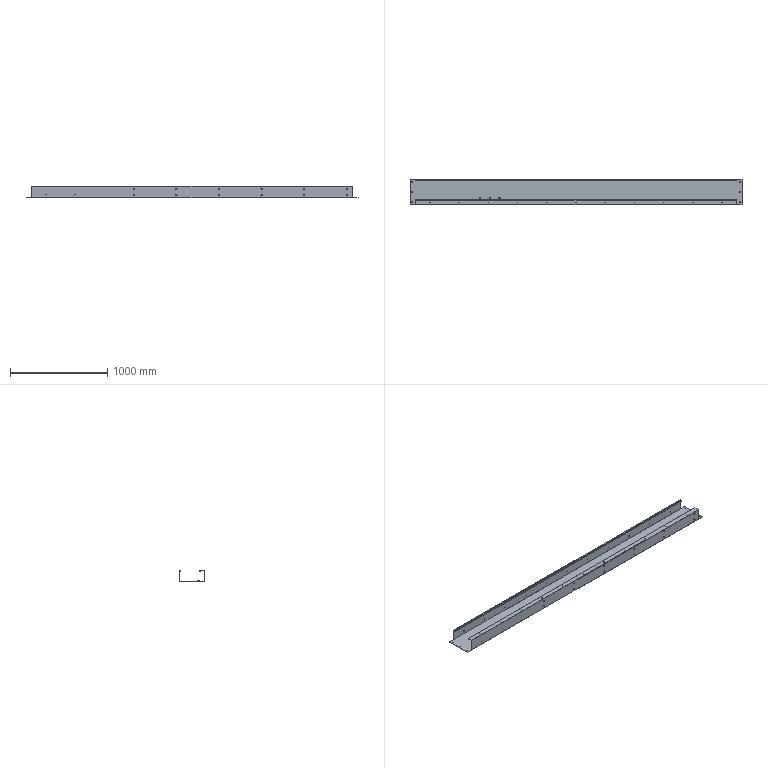Part | STEP file | TS-S28_DefaultSM-FLAT-PATTERN | 1 solid | 239 faces | box 3411 x 262 x 122 mm | volume 3915643 mm3 | cylinder 138 | plane 89 | cone 12 | commonest cylinder face diameters 5.4 x70 10.5 x24 7 x12 0.4 x6 4.4 x6 5 x6